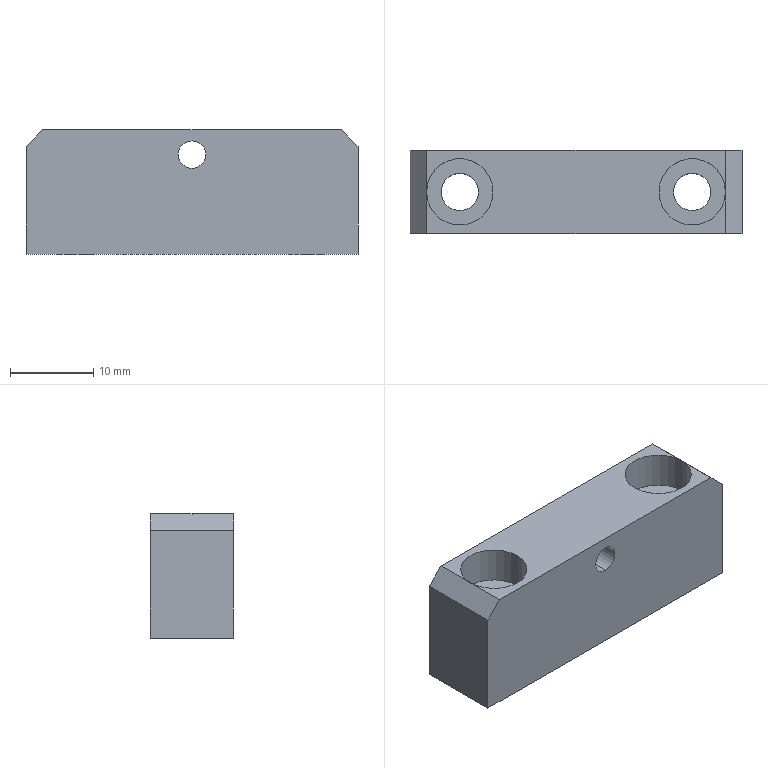Part | STEP file | 11-FG-SZ02011 | 1 solid | 20 faces | box 40 x 10 x 15 mm | volume 5095 mm3 | cylinder 10 | plane 10 | commonest cylinder face diameters 4.5 x4 8 x4 3.3 x2
STEP:
#1=CARTESIAN_POINT('',(0.,-5.,10.35));
#2=VERTEX_POINT('',#1);
#3=CARTESIAN_POINT('',(0.,-5.,13.65));
#4=VERTEX_POINT('',#3);
#5=CARTESIAN_POINT('',(0.,-5.,12.));
#6=DIRECTION('',(0.,1.,0.));
#7=DIRECTION('',(0.,0.,1.));
#8=AXIS2_PLACEMENT_3D('',#5,#6,#7);
#9=CIRCLE('',#8,1.65);
#10=EDGE_CURVE('',#2,#4,#9,.T.);
#11=ORIENTED_EDGE('',*,*,#10,.F.);
#12=CARTESIAN_POINT('',(0.,5.,10.35));
#13=VERTEX_POINT('',#12);
#14=CARTESIAN_POINT('',(0.,5.,10.35));
#15=DIRECTION('',(0.,1.,0.));
#16=VECTOR('',#15,1000.);
#17=LINE('',#14,#16);
#18=EDGE_CURVE('',#2,#13,#17,.T.);
#19=ORIENTED_EDGE('',*,*,#18,.T.);
#20=CARTESIAN_POINT('',(0.,5.,13.65));
#21=VERTEX_POINT('',#20);
#22=CARTESIAN_POINT('',(0.,5.,12.));
#23=DIRECTION('',(0.,1.,0.));
#24=DIRECTION('',(0.,0.,1.));
#25=AXIS2_PLACEMENT_3D('',#22,#23,#24);
#26=CIRCLE('',#25,1.65);
#27=EDGE_CURVE('',#13,#21,#26,.T.);
#28=ORIENTED_EDGE('',*,*,#27,.T.);
#29=CARTESIAN_POINT('',(0.,5.,13.65));
#30=DIRECTION('',(0.,1.,0.));
#31=VECTOR('',#30,1000.);
#32=LINE('',#29,#31);
#33=EDGE_CURVE('',#4,#21,#32,.T.);
#34=ORIENTED_EDGE('',*,*,#33,.F.);
#35=EDGE_LOOP('',(#11,#19,#28,#34));
#36=FACE_OUTER_BOUND('',#35,.T.);
#37=CARTESIAN_POINT('',(0.,5.,12.));
#38=DIRECTION('',(0.,1.,0.));
#39=DIRECTION('',(0.,0.,1.));
#40=AXIS2_PLACEMENT_3D('',#37,#38,#39);
#41=CYLINDRICAL_SURFACE('',#40,1.65);
#42=ADVANCED_FACE('',(#36),#41,.F.);
#43=CARTESIAN_POINT('',(-18.,0.,10.6));
#44=VERTEX_POINT('',#43);
#45=CARTESIAN_POINT('',(-10.,0.,10.6));
#46=VERTEX_POINT('',#45);
#47=CARTESIAN_POINT('',(-14.,0.,10.6));
#48=DIRECTION('',(0.,0.,1.));
#49=DIRECTION('',(1.,0.,0.));
#50=AXIS2_PLACEMENT_3D('',#47,#48,#49);
#51=CIRCLE('',#50,4.);
#52=EDGE_CURVE('',#44,#46,#51,.T.);
#53=ORIENTED_EDGE('',*,*,#52,.F.);
#54=CARTESIAN_POINT('',(-18.,0.,15.));
#55=VERTEX_POINT('',#54);
#56=CARTESIAN_POINT('',(-18.,0.,15.));
#57=DIRECTION('',(0.,0.,1.));
#58=VECTOR('',#57,1000.);
#59=LINE('',#56,#58);
#60=EDGE_CURVE('',#44,#55,#59,.T.);
#61=ORIENTED_EDGE('',*,*,#60,.T.);
#62=CARTESIAN_POINT('',(-10.,0.,15.));
#63=VERTEX_POINT('',#62);
#64=CARTESIAN_POINT('',(-14.,0.,15.));
#65=DIRECTION('',(0.,0.,1.));
#66=DIRECTION('',(1.,0.,0.));
#67=AXIS2_PLACEMENT_3D('',#64,#65,#66);
#68=CIRCLE('',#67,4.);
#69=EDGE_CURVE('',#55,#63,#68,.T.);
#70=ORIENTED_EDGE('',*,*,#69,.T.);
#71=CARTESIAN_POINT('',(-10.,0.,15.));
#72=DIRECTION('',(0.,0.,1.));
#73=VECTOR('',#72,1000.);
#74=LINE('',#71,#73);
#75=EDGE_CURVE('',#46,#63,#74,.T.);
#76=ORIENTED_EDGE('',*,*,#75,.F.);
#77=EDGE_LOOP('',(#53,#61,#70,#76));
#78=FACE_OUTER_BOUND('',#77,.T.);
#79=CARTESIAN_POINT('',(-14.,0.,15.));
#80=DIRECTION('',(0.,0.,1.));
#81=DIRECTION('',(1.,0.,0.));
#82=AXIS2_PLACEMENT_3D('',#79,#80,#81);
#83=CYLINDRICAL_SURFACE('',#82,4.);
#84=ADVANCED_FACE('',(#78),#83,.F.);
#85=CARTESIAN_POINT('',(-16.25,0.,0.));
#86=VERTEX_POINT('',#85);
#87=CARTESIAN_POINT('',(-11.75,0.,0.));
#88=VERTEX_POINT('',#87);
#89=CARTESIAN_POINT('',(-14.,0.,0.));
#90=DIRECTION('',(0.,0.,1.));
#91=DIRECTION('',(1.,0.,0.));
#92=AXIS2_PLACEMENT_3D('',#89,#90,#91);
#93=CIRCLE('',#92,2.25);
#94=EDGE_CURVE('',#86,#88,#93,.T.);
#95=ORIENTED_EDGE('',*,*,#94,.F.);
#96=CARTESIAN_POINT('',(-16.25,0.,10.6));
#97=VERTEX_POINT('',#96);
#98=CARTESIAN_POINT('',(-16.25,0.,15.));
#99=DIRECTION('',(0.,0.,1.));
#100=VECTOR('',#99,1000.);
#101=LINE('',#98,#100);
#102=EDGE_CURVE('',#86,#97,#101,.T.);
#103=ORIENTED_EDGE('',*,*,#102,.T.);
#104=CARTESIAN_POINT('',(-11.75,0.,10.6));
#105=VERTEX_POINT('',#104);
#106=CARTESIAN_POINT('',(-14.,0.,10.6));
#107=DIRECTION('',(0.,0.,1.));
#108=DIRECTION('',(1.,0.,0.));
#109=AXIS2_PLACEMENT_3D('',#106,#107,#108);
#110=CIRCLE('',#109,2.25);
#111=EDGE_CURVE('',#97,#105,#110,.T.);
#112=ORIENTED_EDGE('',*,*,#111,.T.);
#113=CARTESIAN_POINT('',(-11.75,0.,15.));
#114=DIRECTION('',(0.,0.,1.));
#115=VECTOR('',#114,1000.);
#116=LINE('',#113,#115);
#117=EDGE_CURVE('',#88,#105,#116,.T.);
#118=ORIENTED_EDGE('',*,*,#117,.F.);
#119=EDGE_LOOP('',(#95,#103,#112,#118));
#120=FACE_OUTER_BOUND('',#119,.T.);
#121=CARTESIAN_POINT('',(-14.,0.,15.));
#122=DIRECTION('',(0.,0.,1.));
#123=DIRECTION('',(1.,0.,0.));
#124=AXIS2_PLACEMENT_3D('',#121,#122,#123);
#125=CYLINDRICAL_SURFACE('',#124,2.25);
#126=ADVANCED_FACE('',(#120),#125,.F.);
#127=CARTESIAN_POINT('',(10.,0.,10.6));
#128=VERTEX_POINT('',#127);
#129=CARTESIAN_POINT('',(18.,0.,10.6));
#130=VERTEX_POINT('',#129);
#131=CARTESIAN_POINT('',(14.,0.,10.6));
#132=DIRECTION('',(0.,0.,1.));
#133=DIRECTION('',(1.,0.,0.));
#134=AXIS2_PLACEMENT_3D('',#131,#132,#133);
#135=CIRCLE('',#134,4.);
#136=EDGE_CURVE('',#128,#130,#135,.T.);
#137=ORIENTED_EDGE('',*,*,#136,.F.);
#138=CARTESIAN_POINT('',(10.,0.,15.));
#139=VERTEX_POINT('',#138);
#140=CARTESIAN_POINT('',(10.,0.,15.));
#141=DIRECTION('',(0.,0.,1.));
#142=VECTOR('',#141,1000.);
#143=LINE('',#140,#142);
#144=EDGE_CURVE('',#128,#139,#143,.T.);
#145=ORIENTED_EDGE('',*,*,#144,.T.);
#146=CARTESIAN_POINT('',(18.,0.,15.));
#147=VERTEX_POINT('',#146);
#148=CARTESIAN_POINT('',(14.,0.,15.));
#149=DIRECTION('',(0.,0.,1.));
#150=DIRECTION('',(1.,0.,0.));
#151=AXIS2_PLACEMENT_3D('',#148,#149,#150);
#152=CIRCLE('',#151,4.);
#153=EDGE_CURVE('',#139,#147,#152,.T.);
#154=ORIENTED_EDGE('',*,*,#153,.T.);
#155=CARTESIAN_POINT('',(18.,0.,15.));
#156=DIRECTION('',(0.,0.,1.));
#157=VECTOR('',#156,1000.);
#158=LINE('',#155,#157);
#159=EDGE_CURVE('',#130,#147,#158,.T.);
#160=ORIENTED_EDGE('',*,*,#159,.F.);
#161=EDGE_LOOP('',(#137,#145,#154,#160));
#162=FACE_OUTER_BOUND('',#161,.T.);
#163=CARTESIAN_POINT('',(14.,0.,15.));
#164=DIRECTION('',(0.,0.,1.));
#165=DIRECTION('',(1.,0.,0.));
#166=AXIS2_PLACEMENT_3D('',#163,#164,#165);
#167=CYLINDRICAL_SURFACE('',#166,4.);
#168=ADVANCED_FACE('',(#162),#167,.F.);
#169=CARTESIAN_POINT('',(11.75,0.,0.));
#170=VERTEX_POINT('',#169);
#171=CARTESIAN_POINT('',(16.25,0.,0.));
#172=VERTEX_POINT('',#171);
#173=CARTESIAN_POINT('',(14.,0.,0.));
#174=DIRECTION('',(0.,0.,1.));
#175=DIRECTION('',(1.,0.,0.));
#176=AXIS2_PLACEMENT_3D('',#173,#174,#175);
#177=CIRCLE('',#176,2.25);
#178=EDGE_CURVE('',#170,#172,#177,.T.);
#179=ORIENTED_EDGE('',*,*,#178,.F.);
#180=CARTESIAN_POINT('',(11.75,0.,10.6));
#181=VERTEX_POINT('',#180);
#182=CARTESIAN_POINT('',(11.75,0.,15.));
#183=DIRECTION('',(0.,0.,1.));
#184=VECTOR('',#183,1000.);
#185=LINE('',#182,#184);
#186=EDGE_CURVE('',#170,#181,#185,.T.);
#187=ORIENTED_EDGE('',*,*,#186,.T.);
#188=CARTESIAN_POINT('',(16.25,0.,10.6));
#189=VERTEX_POINT('',#188);
#190=CARTESIAN_POINT('',(14.,0.,10.6));
#191=DIRECTION('',(0.,0.,1.));
#192=DIRECTION('',(1.,0.,0.));
#193=AXIS2_PLACEMENT_3D('',#190,#191,#192);
#194=CIRCLE('',#193,2.25);
#195=EDGE_CURVE('',#181,#189,#194,.T.);
#196=ORIENTED_EDGE('',*,*,#195,.T.);
#197=CARTESIAN_POINT('',(16.25,0.,15.));
#198=DIRECTION('',(0.,0.,1.));
#199=VECTOR('',#198,1000.);
#200=LINE('',#197,#199);
#201=EDGE_CURVE('',#172,#189,#200,.T.);
#202=ORIENTED_EDGE('',*,*,#201,.F.);
#203=EDGE_LOOP('',(#179,#187,#196,#202));
#204=FACE_OUTER_BOUND('',#203,.T.);
#205=CARTESIAN_POINT('',(14.,0.,15.));
#206=DIRECTION('',(0.,0.,1.));
#207=DIRECTION('',(1.,0.,0.));
#208=AXIS2_PLACEMENT_3D('',#205,#206,#207);
#209=CYLINDRICAL_SURFACE('',#208,2.25);
#210=ADVANCED_FACE('',(#204),#209,.F.);
#211=CARTESIAN_POINT('',(20.,5.,13.));
#212=VERTEX_POINT('',#211);
#213=CARTESIAN_POINT('',(20.,5.,0.));
#214=VERTEX_POINT('',#213);
#215=CARTESIAN_POINT('',(20.,5.,15.));
#216=DIRECTION('',(0.,0.,-1.));
#217=VECTOR('',#216,1000.);
#218=LINE('',#215,#217);
#219=EDGE_CURVE('',#212,#214,#218,.T.);
#220=ORIENTED_EDGE('',*,*,#219,.F.);
#221=CARTESIAN_POINT('',(20.,-5.,13.));
#222=VERTEX_POINT('',#221);
#223=CARTESIAN_POINT('',(20.,-5.,13.));
#224=DIRECTION('',(0.,-1.,0.));
#225=VECTOR('',#224,1000.);
#226=LINE('',#223,#225);
#227=EDGE_CURVE('',#212,#222,#226,.T.);
#228=ORIENTED_EDGE('',*,*,#227,.T.);
#229=CARTESIAN_POINT('',(20.,-5.,0.));
#230=VERTEX_POINT('',#229);
#231=CARTESIAN_POINT('',(20.,-5.,15.));
#232=DIRECTION('',(0.,0.,-1.));
#233=VECTOR('',#232,1000.);
#234=LINE('',#231,#233);
#235=EDGE_CURVE('',#222,#230,#234,.T.);
#236=ORIENTED_EDGE('',*,*,#235,.T.);
#237=CARTESIAN_POINT('',(20.,5.,0.));
#238=DIRECTION('',(0.,1.,0.));
#239=VECTOR('',#238,1000.);
#240=LINE('',#237,#239);
#241=EDGE_CURVE('',#230,#214,#240,.T.);
#242=ORIENTED_EDGE('',*,*,#241,.T.);
#243=EDGE_LOOP('',(#220,#228,#236,#242));
#244=FACE_OUTER_BOUND('',#243,.T.);
#245=CARTESIAN_POINT('',(20.,5.,15.));
#246=DIRECTION('',(-1.,0.,0.));
#247=DIRECTION('',(0.,0.,1.));
#248=AXIS2_PLACEMENT_3D('',#245,#246,#247);
#249=PLANE('',#248);
#250=ADVANCED_FACE('',(#244),#249,.F.);
#251=CARTESIAN_POINT('',(0.,5.,12.));
#252=DIRECTION('',(0.,1.,0.));
#253=DIRECTION('',(0.,0.,1.));
#254=AXIS2_PLACEMENT_3D('',#251,#252,#253);
#255=CIRCLE('',#254,1.65);
#256=EDGE_CURVE('',#21,#13,#255,.T.);
#257=ORIENTED_EDGE('',*,*,#256,.F.);
#258=ORIENTED_EDGE('',*,*,#27,.F.);
#259=EDGE_LOOP('',(#257,#258));
#260=FACE_BOUND('',#259,.T.);
#261=CARTESIAN_POINT('',(18.,5.,15.));
#262=VERTEX_POINT('',#261);
#263=CARTESIAN_POINT('',(-18.,5.,15.));
#264=VERTEX_POINT('',#263);
#265=CARTESIAN_POINT('',(-20.,5.,15.));
#266=DIRECTION('',(-1.,0.,0.));
#267=VECTOR('',#266,1000.);
#268=LINE('',#265,#267);
#269=EDGE_CURVE('',#262,#264,#268,.T.);
#270=ORIENTED_EDGE('',*,*,#269,.F.);
#271=CARTESIAN_POINT('',(18.,5.,15.));
#272=DIRECTION('',(0.7071,0.,-0.7071));
#273=VECTOR('',#272,1000.);
#274=LINE('',#271,#273);
#275=EDGE_CURVE('',#262,#212,#274,.T.);
#276=ORIENTED_EDGE('',*,*,#275,.T.);
#277=ORIENTED_EDGE('',*,*,#219,.T.);
#278=CARTESIAN_POINT('',(-20.,5.,0.));
#279=VERTEX_POINT('',#278);
#280=CARTESIAN_POINT('',(-20.,5.,0.));
#281=DIRECTION('',(-1.,0.,0.));
#282=VECTOR('',#281,1000.);
#283=LINE('',#280,#282);
#284=EDGE_CURVE('',#214,#279,#283,.T.);
#285=ORIENTED_EDGE('',*,*,#284,.T.);
#286=CARTESIAN_POINT('',(-20.,5.,13.));
#287=VERTEX_POINT('',#286);
#288=CARTESIAN_POINT('',(-20.,5.,15.));
#289=DIRECTION('',(0.,0.,-1.));
#290=VECTOR('',#289,1000.);
#291=LINE('',#288,#290);
#292=EDGE_CURVE('',#287,#279,#291,.T.);
#293=ORIENTED_EDGE('',*,*,#292,.F.);
#294=CARTESIAN_POINT('',(-18.,5.,15.));
#295=DIRECTION('',(0.7071,0.,0.7071));
#296=VECTOR('',#295,1000.);
#297=LINE('',#294,#296);
#298=EDGE_CURVE('',#287,#264,#297,.T.);
#299=ORIENTED_EDGE('',*,*,#298,.T.);
#300=EDGE_LOOP('',(#270,#276,#277,#285,#293,#299));
#301=FACE_OUTER_BOUND('',#300,.T.);
#302=CARTESIAN_POINT('',(-20.,5.,15.));
#303=DIRECTION('',(0.,-1.,0.));
#304=DIRECTION('',(0.,0.,-1.));
#305=AXIS2_PLACEMENT_3D('',#302,#303,#304);
#306=PLANE('',#305);
#307=ADVANCED_FACE('',(#260,#301),#306,.F.);
#308=CARTESIAN_POINT('',(-20.,-5.,13.));
#309=VERTEX_POINT('',#308);
#310=CARTESIAN_POINT('',(-20.,-5.,0.));
#311=VERTEX_POINT('',#310);
#312=CARTESIAN_POINT('',(-20.,-5.,15.));
#313=DIRECTION('',(0.,0.,-1.));
#314=VECTOR('',#313,1000.);
#315=LINE('',#312,#314);
#316=EDGE_CURVE('',#309,#311,#315,.T.);
#317=ORIENTED_EDGE('',*,*,#316,.F.);
#318=CARTESIAN_POINT('',(-20.,5.,13.));
#319=DIRECTION('',(0.,1.,0.));
#320=VECTOR('',#319,1000.);
#321=LINE('',#318,#320);
#322=EDGE_CURVE('',#309,#287,#321,.T.);
#323=ORIENTED_EDGE('',*,*,#322,.T.);
#324=ORIENTED_EDGE('',*,*,#292,.T.);
#325=CARTESIAN_POINT('',(-20.,5.,0.));
#326=DIRECTION('',(0.,-1.,0.));
#327=VECTOR('',#326,1000.);
#328=LINE('',#325,#327);
#329=EDGE_CURVE('',#279,#311,#328,.T.);
#330=ORIENTED_EDGE('',*,*,#329,.T.);
#331=EDGE_LOOP('',(#317,#323,#324,#330));
#332=FACE_OUTER_BOUND('',#331,.T.);
#333=CARTESIAN_POINT('',(-20.,5.,15.));
#334=DIRECTION('',(1.,0.,0.));
#335=DIRECTION('',(0.,0.,-1.));
#336=AXIS2_PLACEMENT_3D('',#333,#334,#335);
#337=PLANE('',#336);
#338=ADVANCED_FACE('',(#332),#337,.F.);
#339=CARTESIAN_POINT('',(0.,-5.,12.));
#340=DIRECTION('',(0.,1.,0.));
#341=DIRECTION('',(0.,0.,1.));
#342=AXIS2_PLACEMENT_3D('',#339,#340,#341);
#343=CIRCLE('',#342,1.65);
#344=EDGE_CURVE('',#4,#2,#343,.T.);
#345=ORIENTED_EDGE('',*,*,#344,.T.);
#346=ORIENTED_EDGE('',*,*,#10,.T.);
#347=EDGE_LOOP('',(#345,#346));
#348=FACE_BOUND('',#347,.T.);
#349=ORIENTED_EDGE('',*,*,#235,.F.);
#350=CARTESIAN_POINT('',(18.,-5.,15.));
#351=VERTEX_POINT('',#350);
#352=CARTESIAN_POINT('',(18.,-5.,15.));
#353=DIRECTION('',(-0.7071,0.,0.7071));
#354=VECTOR('',#353,1000.);
#355=LINE('',#352,#354);
#356=EDGE_CURVE('',#222,#351,#355,.T.);
#357=ORIENTED_EDGE('',*,*,#356,.T.);
#358=CARTESIAN_POINT('',(-18.,-5.,15.));
#359=VERTEX_POINT('',#358);
#360=CARTESIAN_POINT('',(-20.,-5.,15.));
#361=DIRECTION('',(1.,0.,0.));
#362=VECTOR('',#361,1000.);
#363=LINE('',#360,#362);
#364=EDGE_CURVE('',#359,#351,#363,.T.);
#365=ORIENTED_EDGE('',*,*,#364,.F.);
#366=CARTESIAN_POINT('',(-18.,-5.,15.));
#367=DIRECTION('',(-0.7071,0.,-0.7071));
#368=VECTOR('',#367,1000.);
#369=LINE('',#366,#368);
#370=EDGE_CURVE('',#359,#309,#369,.T.);
#371=ORIENTED_EDGE('',*,*,#370,.T.);
#372=ORIENTED_EDGE('',*,*,#316,.T.);
#373=CARTESIAN_POINT('',(-20.,-5.,0.));
#374=DIRECTION('',(1.,0.,0.));
#375=VECTOR('',#374,1000.);
#376=LINE('',#373,#375);
#377=EDGE_CURVE('',#311,#230,#376,.T.);
#378=ORIENTED_EDGE('',*,*,#377,.T.);
#379=EDGE_LOOP('',(#349,#357,#365,#371,#372,#378));
#380=FACE_OUTER_BOUND('',#379,.T.);
#381=CARTESIAN_POINT('',(-20.,-5.,15.));
#382=DIRECTION('',(0.,1.,0.));
#383=DIRECTION('',(0.,0.,1.));
#384=AXIS2_PLACEMENT_3D('',#381,#382,#383);
#385=PLANE('',#384);
#386=ADVANCED_FACE('',(#348,#380),#385,.F.);
#387=ORIENTED_EDGE('',*,*,#364,.T.);
#388=CARTESIAN_POINT('',(18.,5.,15.));
#389=DIRECTION('',(0.,1.,0.));
#390=VECTOR('',#389,1000.);
#391=LINE('',#388,#390);
#392=EDGE_CURVE('',#351,#147,#391,.T.);
#393=ORIENTED_EDGE('',*,*,#392,.T.);
#394=ORIENTED_EDGE('',*,*,#153,.F.);
#395=CARTESIAN_POINT('',(14.,0.,15.));
#396=DIRECTION('',(0.,0.,1.));
#397=DIRECTION('',(1.,0.,0.));
#398=AXIS2_PLACEMENT_3D('',#395,#396,#397);
#399=CIRCLE('',#398,4.);
#400=EDGE_CURVE('',#147,#139,#399,.T.);
#401=ORIENTED_EDGE('',*,*,#400,.F.);
#402=CARTESIAN_POINT('',(18.,5.,15.));
#403=DIRECTION('',(0.,1.,0.));
#404=VECTOR('',#403,1000.);
#405=LINE('',#402,#404);
#406=EDGE_CURVE('',#147,#262,#405,.T.);
#407=ORIENTED_EDGE('',*,*,#406,.T.);
#408=ORIENTED_EDGE('',*,*,#269,.T.);
#409=CARTESIAN_POINT('',(-18.,-5.,15.));
#410=DIRECTION('',(0.,-1.,0.));
#411=VECTOR('',#410,1000.);
#412=LINE('',#409,#411);
#413=EDGE_CURVE('',#264,#55,#412,.T.);
#414=ORIENTED_EDGE('',*,*,#413,.T.);
#415=CARTESIAN_POINT('',(-14.,0.,15.));
#416=DIRECTION('',(0.,0.,1.));
#417=DIRECTION('',(1.,0.,0.));
#418=AXIS2_PLACEMENT_3D('',#415,#416,#417);
#419=CIRCLE('',#418,4.);
#420=EDGE_CURVE('',#63,#55,#419,.T.);
#421=ORIENTED_EDGE('',*,*,#420,.F.);
#422=ORIENTED_EDGE('',*,*,#69,.F.);
#423=CARTESIAN_POINT('',(-18.,-5.,15.));
#424=DIRECTION('',(0.,-1.,0.));
#425=VECTOR('',#424,1000.);
#426=LINE('',#423,#425);
#427=EDGE_CURVE('',#55,#359,#426,.T.);
#428=ORIENTED_EDGE('',*,*,#427,.T.);
#429=EDGE_LOOP('',(#387,#393,#394,#401,#407,#408,#414,#421,#422,#428));
#430=FACE_OUTER_BOUND('',#429,.T.);
#431=CARTESIAN_POINT('',(0.,0.,15.));
#432=DIRECTION('',(0.,0.,1.));
#433=DIRECTION('',(1.,0.,0.));
#434=AXIS2_PLACEMENT_3D('',#431,#432,#433);
#435=PLANE('',#434);
#436=ADVANCED_FACE('',(#430),#435,.T.);
#437=CARTESIAN_POINT('',(-14.,0.,0.));
#438=DIRECTION('',(0.,0.,1.));
#439=DIRECTION('',(1.,0.,0.));
#440=AXIS2_PLACEMENT_3D('',#437,#438,#439);
#441=CIRCLE('',#440,2.25);
#442=EDGE_CURVE('',#88,#86,#441,.T.);
#443=ORIENTED_EDGE('',*,*,#442,.T.);
#444=ORIENTED_EDGE('',*,*,#94,.T.);
#445=EDGE_LOOP('',(#443,#444));
#446=FACE_BOUND('',#445,.T.);
#447=CARTESIAN_POINT('',(14.,0.,0.));
#448=DIRECTION('',(0.,0.,1.));
#449=DIRECTION('',(1.,0.,0.));
#450=AXIS2_PLACEMENT_3D('',#447,#448,#449);
#451=CIRCLE('',#450,2.25);
#452=EDGE_CURVE('',#172,#170,#451,.T.);
#453=ORIENTED_EDGE('',*,*,#452,.T.);
#454=ORIENTED_EDGE('',*,*,#178,.T.);
#455=EDGE_LOOP('',(#453,#454));
#456=FACE_BOUND('',#455,.T.);
#457=ORIENTED_EDGE('',*,*,#241,.F.);
#458=ORIENTED_EDGE('',*,*,#377,.F.);
#459=ORIENTED_EDGE('',*,*,#329,.F.);
#460=ORIENTED_EDGE('',*,*,#284,.F.);
#461=EDGE_LOOP('',(#457,#458,#459,#460));
#462=FACE_OUTER_BOUND('',#461,.T.);
#463=CARTESIAN_POINT('',(0.,0.,0.));
#464=DIRECTION('',(0.,0.,1.));
#465=DIRECTION('',(1.,0.,0.));
#466=AXIS2_PLACEMENT_3D('',#463,#464,#465);
#467=PLANE('',#466);
#468=ADVANCED_FACE('',(#446,#456,#462),#467,.F.);
#469=ORIENTED_EDGE('',*,*,#186,.F.);
#470=ORIENTED_EDGE('',*,*,#452,.F.);
#471=ORIENTED_EDGE('',*,*,#201,.T.);
#472=CARTESIAN_POINT('',(14.,0.,10.6));
#473=DIRECTION('',(0.,0.,1.));
#474=DIRECTION('',(1.,0.,0.));
#475=AXIS2_PLACEMENT_3D('',#472,#473,#474);
#476=CIRCLE('',#475,2.25);
#477=EDGE_CURVE('',#189,#181,#476,.T.);
#478=ORIENTED_EDGE('',*,*,#477,.T.);
#479=EDGE_LOOP('',(#469,#470,#471,#478));
#480=FACE_OUTER_BOUND('',#479,.T.);
#481=CARTESIAN_POINT('',(14.,0.,15.));
#482=DIRECTION('',(0.,0.,1.));
#483=DIRECTION('',(1.,0.,0.));
#484=AXIS2_PLACEMENT_3D('',#481,#482,#483);
#485=CYLINDRICAL_SURFACE('',#484,2.25);
#486=ADVANCED_FACE('',(#480),#485,.F.);
#487=ORIENTED_EDGE('',*,*,#477,.F.);
#488=ORIENTED_EDGE('',*,*,#195,.F.);
#489=EDGE_LOOP('',(#487,#488));
#490=FACE_BOUND('',#489,.T.);
#491=CARTESIAN_POINT('',(14.,0.,10.6));
#492=DIRECTION('',(0.,0.,1.));
#493=DIRECTION('',(1.,0.,0.));
#494=AXIS2_PLACEMENT_3D('',#491,#492,#493);
#495=CIRCLE('',#494,4.);
#496=EDGE_CURVE('',#130,#128,#495,.T.);
#497=ORIENTED_EDGE('',*,*,#496,.T.);
#498=ORIENTED_EDGE('',*,*,#136,.T.);
#499=EDGE_LOOP('',(#497,#498));
#500=FACE_OUTER_BOUND('',#499,.T.);
#501=CARTESIAN_POINT('',(16.25,0.,10.6));
#502=DIRECTION('',(0.,0.,-1.));
#503=DIRECTION('',(-1.,0.,0.));
#504=AXIS2_PLACEMENT_3D('',#501,#502,#503);
#505=PLANE('',#504);
#506=ADVANCED_FACE('',(#490,#500),#505,.F.);
#507=ORIENTED_EDGE('',*,*,#144,.F.);
#508=ORIENTED_EDGE('',*,*,#496,.F.);
#509=ORIENTED_EDGE('',*,*,#159,.T.);
#510=ORIENTED_EDGE('',*,*,#400,.T.);
#511=EDGE_LOOP('',(#507,#508,#509,#510));
#512=FACE_OUTER_BOUND('',#511,.T.);
#513=CARTESIAN_POINT('',(14.,0.,15.));
#514=DIRECTION('',(0.,0.,1.));
#515=DIRECTION('',(1.,0.,0.));
#516=AXIS2_PLACEMENT_3D('',#513,#514,#515);
#517=CYLINDRICAL_SURFACE('',#516,4.);
#518=ADVANCED_FACE('',(#512),#517,.F.);
#519=ORIENTED_EDGE('',*,*,#102,.F.);
#520=ORIENTED_EDGE('',*,*,#442,.F.);
#521=ORIENTED_EDGE('',*,*,#117,.T.);
#522=CARTESIAN_POINT('',(-14.,0.,10.6));
#523=DIRECTION('',(0.,0.,1.));
#524=DIRECTION('',(1.,0.,0.));
#525=AXIS2_PLACEMENT_3D('',#522,#523,#524);
#526=CIRCLE('',#525,2.25);
#527=EDGE_CURVE('',#105,#97,#526,.T.);
#528=ORIENTED_EDGE('',*,*,#527,.T.);
#529=EDGE_LOOP('',(#519,#520,#521,#528));
#530=FACE_OUTER_BOUND('',#529,.T.);
#531=CARTESIAN_POINT('',(-14.,0.,15.));
#532=DIRECTION('',(0.,0.,1.));
#533=DIRECTION('',(1.,0.,0.));
#534=AXIS2_PLACEMENT_3D('',#531,#532,#533);
#535=CYLINDRICAL_SURFACE('',#534,2.25);
#536=ADVANCED_FACE('',(#530),#535,.F.);
#537=ORIENTED_EDGE('',*,*,#527,.F.);
#538=ORIENTED_EDGE('',*,*,#111,.F.);
#539=EDGE_LOOP('',(#537,#538));
#540=FACE_BOUND('',#539,.T.);
#541=CARTESIAN_POINT('',(-14.,0.,10.6));
#542=DIRECTION('',(0.,0.,1.));
#543=DIRECTION('',(1.,0.,0.));
#544=AXIS2_PLACEMENT_3D('',#541,#542,#543);
#545=CIRCLE('',#544,4.);
#546=EDGE_CURVE('',#46,#44,#545,.T.);
#547=ORIENTED_EDGE('',*,*,#546,.T.);
#548=ORIENTED_EDGE('',*,*,#52,.T.);
#549=EDGE_LOOP('',(#547,#548));
#550=FACE_OUTER_BOUND('',#549,.T.);
#551=CARTESIAN_POINT('',(-11.75,0.,10.6));
#552=DIRECTION('',(0.,0.,-1.));
#553=DIRECTION('',(-1.,0.,0.));
#554=AXIS2_PLACEMENT_3D('',#551,#552,#553);
#555=PLANE('',#554);
#556=ADVANCED_FACE('',(#540,#550),#555,.F.);
#557=ORIENTED_EDGE('',*,*,#60,.F.);
#558=ORIENTED_EDGE('',*,*,#546,.F.);
#559=ORIENTED_EDGE('',*,*,#75,.T.);
#560=ORIENTED_EDGE('',*,*,#420,.T.);
#561=EDGE_LOOP('',(#557,#558,#559,#560));
#562=FACE_OUTER_BOUND('',#561,.T.);
#563=CARTESIAN_POINT('',(-14.,0.,15.));
#564=DIRECTION('',(0.,0.,1.));
#565=DIRECTION('',(1.,0.,0.));
#566=AXIS2_PLACEMENT_3D('',#563,#564,#565);
#567=CYLINDRICAL_SURFACE('',#566,4.);
#568=ADVANCED_FACE('',(#562),#567,.F.);
#569=ORIENTED_EDGE('',*,*,#18,.F.);
#570=ORIENTED_EDGE('',*,*,#344,.F.);
#571=ORIENTED_EDGE('',*,*,#33,.T.);
#572=ORIENTED_EDGE('',*,*,#256,.T.);
#573=EDGE_LOOP('',(#569,#570,#571,#572));
#574=FACE_OUTER_BOUND('',#573,.T.);
#575=CARTESIAN_POINT('',(0.,5.,12.));
#576=DIRECTION('',(0.,1.,0.));
#577=DIRECTION('',(0.,0.,1.));
#578=AXIS2_PLACEMENT_3D('',#575,#576,#577);
#579=CYLINDRICAL_SURFACE('',#578,1.65);
#580=ADVANCED_FACE('',(#574),#579,.F.);
#581=ORIENTED_EDGE('',*,*,#356,.F.);
#582=ORIENTED_EDGE('',*,*,#227,.F.);
#583=ORIENTED_EDGE('',*,*,#275,.F.);
#584=ORIENTED_EDGE('',*,*,#406,.F.);
#585=ORIENTED_EDGE('',*,*,#392,.F.);
#586=EDGE_LOOP('',(#581,#582,#583,#584,#585));
#587=FACE_OUTER_BOUND('',#586,.T.);
#588=CARTESIAN_POINT('',(18.,0.,15.));
#589=DIRECTION('',(0.7071,0.,0.7071));
#590=DIRECTION('',(0.,-1.,0.));
#591=AXIS2_PLACEMENT_3D('',#588,#589,#590);
#592=PLANE('',#591);
#593=ADVANCED_FACE('',(#587),#592,.T.);
#594=ORIENTED_EDGE('',*,*,#298,.F.);
#595=ORIENTED_EDGE('',*,*,#322,.F.);
#596=ORIENTED_EDGE('',*,*,#370,.F.);
#597=ORIENTED_EDGE('',*,*,#427,.F.);
#598=ORIENTED_EDGE('',*,*,#413,.F.);
#599=EDGE_LOOP('',(#594,#595,#596,#597,#598));
#600=FACE_OUTER_BOUND('',#599,.T.);
#601=CARTESIAN_POINT('',(-18.,0.,15.));
#602=DIRECTION('',(-0.7071,0.,0.7071));
#603=DIRECTION('',(0.,1.,0.));
#604=AXIS2_PLACEMENT_3D('',#601,#602,#603);
#605=PLANE('',#604);
#606=ADVANCED_FACE('',(#600),#605,.T.);
#607=CLOSED_SHELL('',(#42,#84,#126,#168,#210,#250,#307,#338,#386,#436,#468,#486,#506,#518,#536,#556,#568,#580,#593,#606));
#608=MANIFOLD_SOLID_BREP('',#607);
#609=CARTESIAN_POINT('',(0.,0.,0.));
#610=DIRECTION('',(0.,0.,1.));
#611=DIRECTION('',(1.,0.,0.));
#612=AXIS2_PLACEMENT_3D('',#609,#610,#611);
#613=(LENGTH_UNIT()NAMED_UNIT(*)SI_UNIT(.MILLI.,.METRE.));
#614=UNCERTAINTY_MEASURE_WITH_UNIT(LENGTH_MEASURE(0.00001),#613,'','');
#615=(NAMED_UNIT(*)PLANE_ANGLE_UNIT()SI_UNIT($,.RADIAN.));
#616=(NAMED_UNIT(*)SI_UNIT($,.STERADIAN.)SOLID_ANGLE_UNIT());
#617=(GEOMETRIC_REPRESENTATION_CONTEXT(3)GLOBAL_UNCERTAINTY_ASSIGNED_CONTEXT((#614))GLOBAL_UNIT_ASSIGNED_CONTEXT((#613,#615,#616))REPRESENTATION_CONTEXT('',''));
#618=ADVANCED_BREP_SHAPE_REPRESENTATION('',(#608,#612),#617);